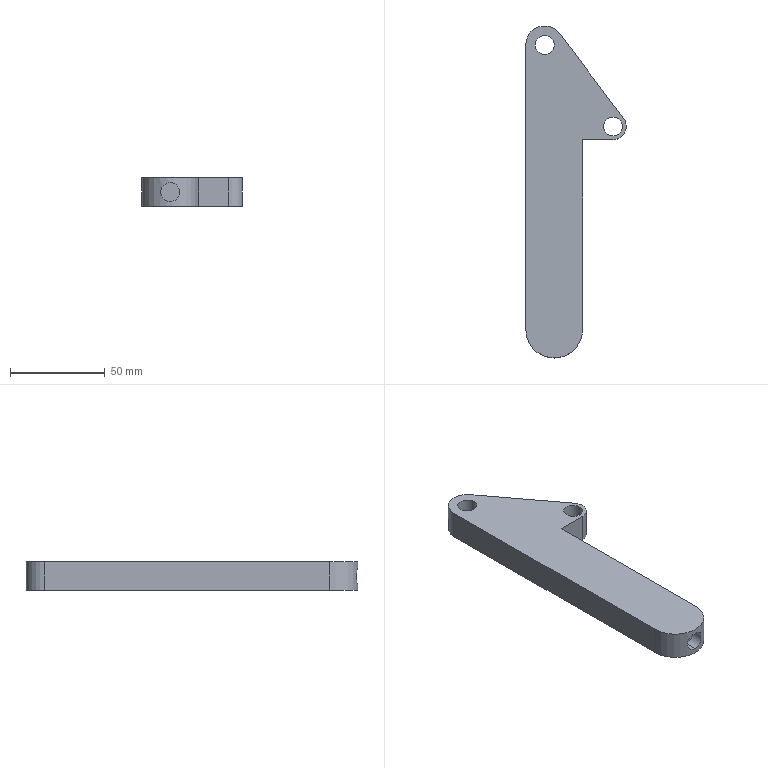Part | STEP file | 1 solid | 20 faces | box 53 x 175 x 15 mm | volume 79206 mm3 | cylinder 12 | plane 8 | commonest cylinder face diameters 10 x8 14 x2 20 x1 30 x1